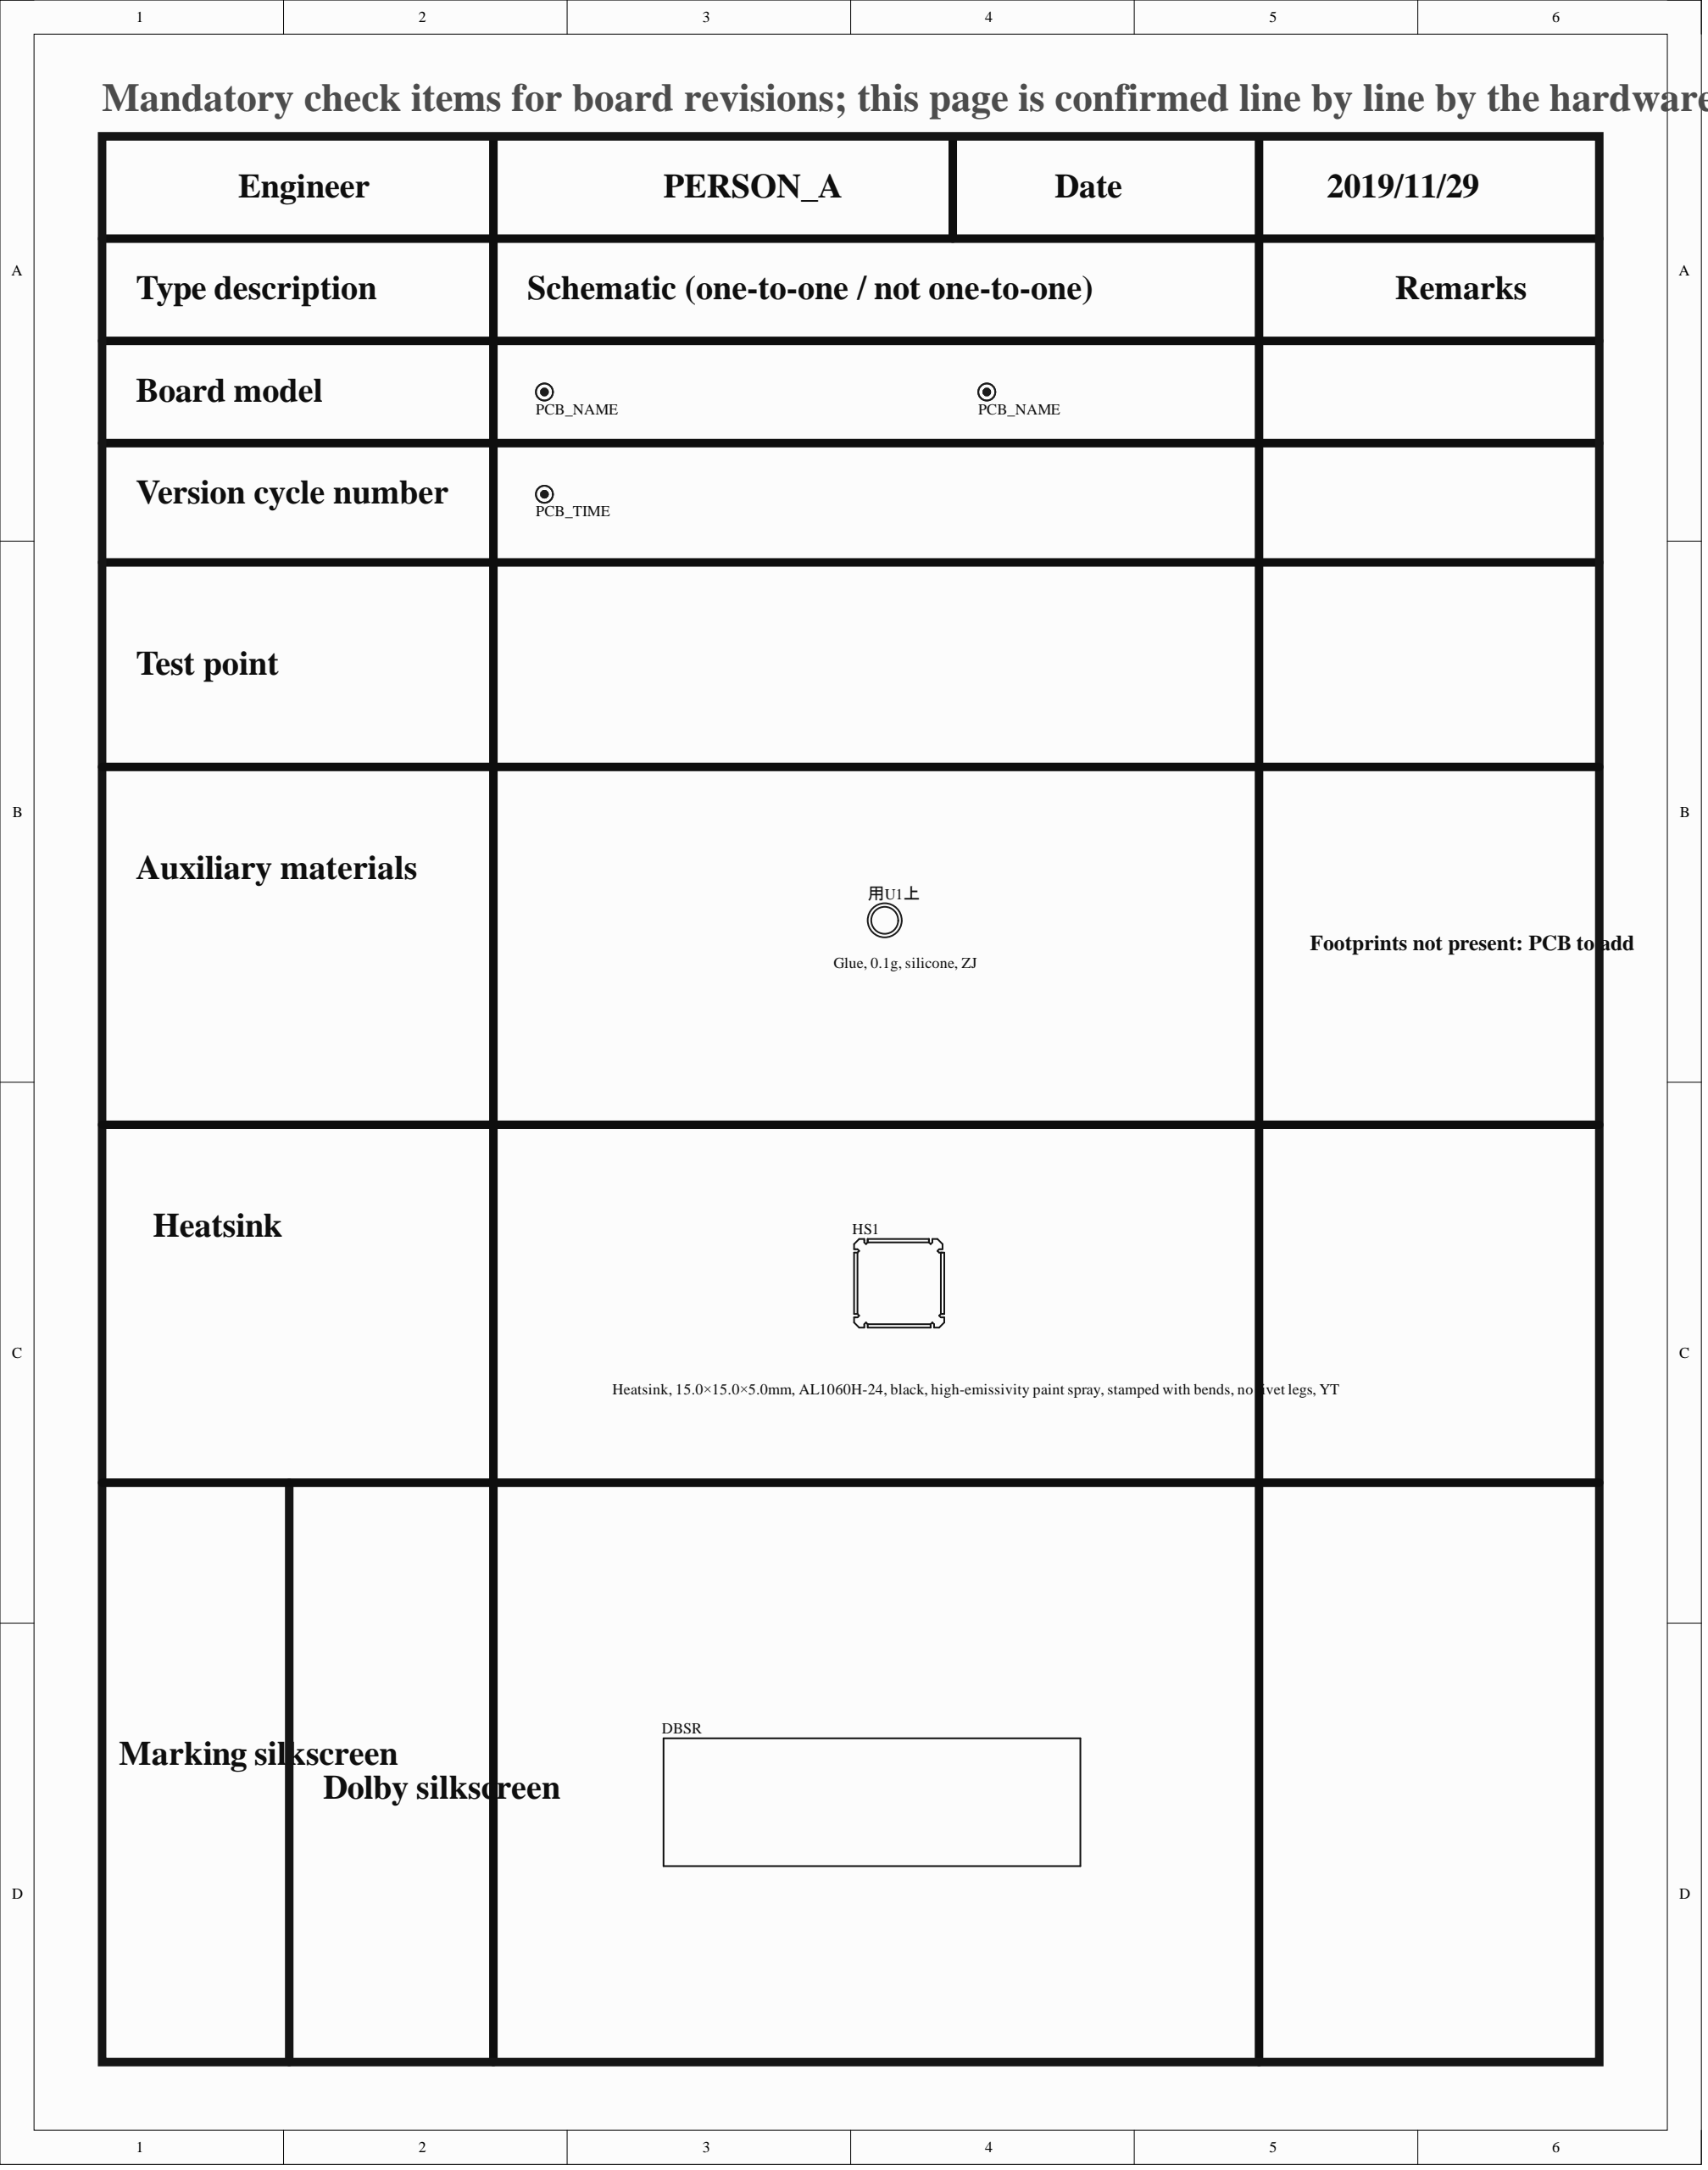Circuit board | Altium Designer | 541 parts | 263 nets | one sheet of the schematic
Parts on this sheet (reference | value | footprint):
DBSR | NO DOLBY | NO DOLBY-SILK
HS1 | Heatsink, 15.0×15.0×5.0mm, AL1060H-24, black, high-emissivity paint spray, stamped with bends, no rivet legs, YT | HS(15X15X5)-S
用U1上 | Glue, 0.1g, silicone, ZJ | Heat-Shrinkable Tube
Nets of these parts (net: part-pin ...):